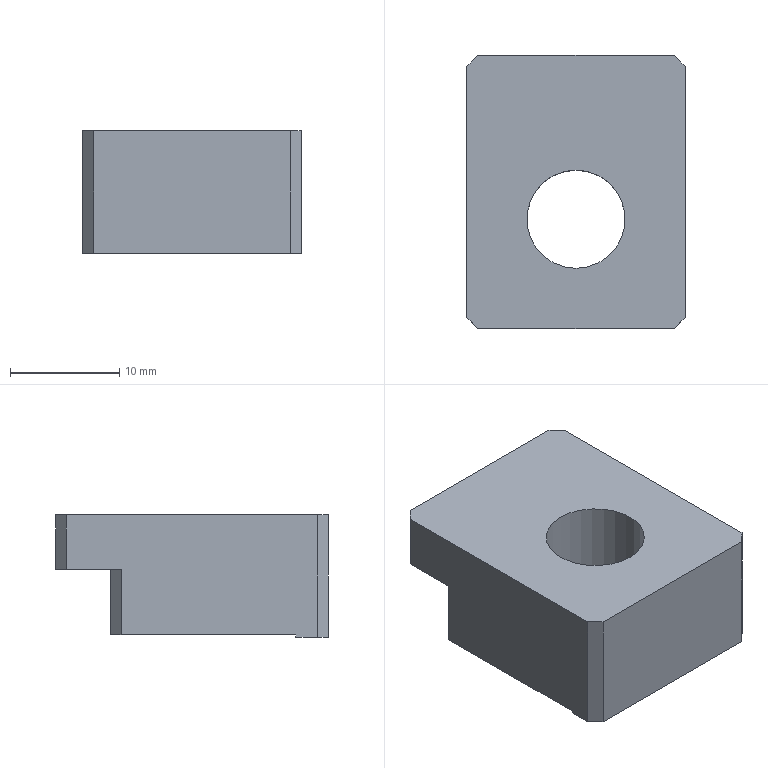Part | NX | features solid 2 | 1 solid | 17 faces | box 20 x 25 x 11.2 mm | volume 4190 mm3 | plane 16 | cylinder 1 | commonest cylinder face diameters 9 x1
STEP:
#1=CARTESIAN_POINT('',(146.5,-346.,61.));
#2=VERTEX_POINT('',#1);
#3=CARTESIAN_POINT('',(146.5,-350.5,61.));
#4=DIRECTION('',(0.,0.,-1.));
#5=DIRECTION('',(0.,1.,0.));
#6=AXIS2_PLACEMENT_3D('',#3,#4,#5);
#7=CIRCLE('',#6,4.5);
#8=EDGE_CURVE('',#2,#2,#7,.T.);
#9=ORIENTED_EDGE('',*,*,#8,.F.);
#10=EDGE_LOOP('',(#9));
#11=FACE_BOUND('',#10,.T.);
#12=CARTESIAN_POINT('',(146.5,-355.,50.));
#13=VERTEX_POINT('',#12);
#14=CARTESIAN_POINT('',(146.5,-350.5,50.));
#15=DIRECTION('',(0.,0.,1.));
#16=DIRECTION('',(0.,-1.,0.));
#17=AXIS2_PLACEMENT_3D('',#14,#15,#16);
#18=CIRCLE('',#17,4.5);
#19=EDGE_CURVE('',#13,#13,#18,.T.);
#20=ORIENTED_EDGE('',*,*,#19,.F.);
#21=EDGE_LOOP('',(#20));
#22=FACE_BOUND('',#21,.T.);
#23=CARTESIAN_POINT('',(146.5,-350.5,10.));
#24=DIRECTION('',(0.,0.,-1.));
#25=DIRECTION('',(0.,1.,0.));
#26=AXIS2_PLACEMENT_3D('',#23,#24,#25);
#27=CYLINDRICAL_SURFACE('',#26,4.5);
#28=ADVANCED_FACE('',(#11,#22),#27,.F.);
#29=CARTESIAN_POINT('',(155.5,-335.5,61.));
#30=VERTEX_POINT('',#29);
#31=CARTESIAN_POINT('',(137.5,-335.5,61.));
#32=VERTEX_POINT('',#31);
#33=CARTESIAN_POINT('',(177.825,-335.5,61.));
#34=DIRECTION('',(-1.,0.,0.));
#35=VECTOR('',#34,1000.);
#36=LINE('',#33,#35);
#37=EDGE_CURVE('',#30,#32,#36,.T.);
#38=ORIENTED_EDGE('',*,*,#37,.T.);
#39=CARTESIAN_POINT('',(136.5,-336.5,61.));
#40=VERTEX_POINT('',#39);
#41=CARTESIAN_POINT('',(137.5,-335.5,61.));
#42=DIRECTION('',(-0.7071,-0.7071,0.));
#43=VECTOR('',#42,1000.);
#44=LINE('',#41,#43);
#45=EDGE_CURVE('',#32,#40,#44,.T.);
#46=ORIENTED_EDGE('',*,*,#45,.T.);
#47=CARTESIAN_POINT('',(136.5,-359.5,61.));
#48=VERTEX_POINT('',#47);
#49=CARTESIAN_POINT('',(136.5,-323.825,61.));
#50=DIRECTION('',(0.,1.,0.));
#51=VECTOR('',#50,1000.);
#52=LINE('',#49,#51);
#53=EDGE_CURVE('',#48,#40,#52,.T.);
#54=ORIENTED_EDGE('',*,*,#53,.F.);
#55=CARTESIAN_POINT('',(137.5,-360.5,61.));
#56=VERTEX_POINT('',#55);
#57=CARTESIAN_POINT('',(136.5,-359.5,61.));
#58=DIRECTION('',(0.7071,-0.7071,0.));
#59=VECTOR('',#58,1000.);
#60=LINE('',#57,#59);
#61=EDGE_CURVE('',#48,#56,#60,.T.);
#62=ORIENTED_EDGE('',*,*,#61,.T.);
#63=CARTESIAN_POINT('',(155.5,-360.5,61.));
#64=VERTEX_POINT('',#63);
#65=CARTESIAN_POINT('',(177.825,-360.5,61.));
#66=DIRECTION('',(1.,0.,0.));
#67=VECTOR('',#66,1000.);
#68=LINE('',#65,#67);
#69=EDGE_CURVE('',#56,#64,#68,.T.);
#70=ORIENTED_EDGE('',*,*,#69,.T.);
#71=CARTESIAN_POINT('',(156.5,-359.5,61.));
#72=VERTEX_POINT('',#71);
#73=CARTESIAN_POINT('',(155.5,-360.5,61.));
#74=DIRECTION('',(0.7071,0.7071,0.));
#75=VECTOR('',#74,1000.);
#76=LINE('',#73,#75);
#77=EDGE_CURVE('',#64,#72,#76,.T.);
#78=ORIENTED_EDGE('',*,*,#77,.T.);
#79=CARTESIAN_POINT('',(156.5,-336.5,61.));
#80=VERTEX_POINT('',#79);
#81=CARTESIAN_POINT('',(156.5,-323.825,61.));
#82=DIRECTION('',(0.,1.,0.));
#83=VECTOR('',#82,1000.);
#84=LINE('',#81,#83);
#85=EDGE_CURVE('',#72,#80,#84,.T.);
#86=ORIENTED_EDGE('',*,*,#85,.T.);
#87=CARTESIAN_POINT('',(155.5,-335.5,61.));
#88=DIRECTION('',(-0.7071,0.7071,0.));
#89=VECTOR('',#88,1000.);
#90=LINE('',#87,#89);
#91=EDGE_CURVE('',#80,#30,#90,.T.);
#92=ORIENTED_EDGE('',*,*,#91,.T.);
#93=EDGE_LOOP('',(#38,#46,#54,#62,#70,#78,#86,#92));
#94=FACE_BOUND('',#93,.T.);
#95=ORIENTED_EDGE('',*,*,#8,.T.);
#96=EDGE_LOOP('',(#95));
#97=FACE_BOUND('',#96,.T.);
#98=CARTESIAN_POINT('',(177.825,-323.825,61.));
#99=DIRECTION('',(0.,0.,-1.));
#100=DIRECTION('',(-0.7071,0.7071,0.));
#101=AXIS2_PLACEMENT_3D('',#98,#99,#100);
#102=PLANE('',#101);
#103=ADVANCED_FACE('',(#94,#97),#102,.F.);
#104=ORIENTED_EDGE('',*,*,#91,.F.);
#105=CARTESIAN_POINT('',(156.5,-336.5,56.));
#106=VERTEX_POINT('',#105);
#107=CARTESIAN_POINT('',(156.5,-336.5,57.5));
#108=DIRECTION('',(0.,0.,1.));
#109=VECTOR('',#108,1000.);
#110=LINE('',#107,#109);
#111=EDGE_CURVE('',#106,#80,#110,.T.);
#112=ORIENTED_EDGE('',*,*,#111,.F.);
#113=CARTESIAN_POINT('',(155.5,-335.5,56.));
#114=VERTEX_POINT('',#113);
#115=CARTESIAN_POINT('',(155.5,-335.5,56.));
#116=DIRECTION('',(0.7071,-0.7071,0.));
#117=VECTOR('',#116,1000.);
#118=LINE('',#115,#117);
#119=EDGE_CURVE('',#114,#106,#118,.T.);
#120=ORIENTED_EDGE('',*,*,#119,.F.);
#121=CARTESIAN_POINT('',(155.5,-335.5,60.));
#122=DIRECTION('',(0.,0.,-1.));
#123=VECTOR('',#122,1000.);
#124=LINE('',#121,#123);
#125=EDGE_CURVE('',#30,#114,#124,.T.);
#126=ORIENTED_EDGE('',*,*,#125,.F.);
#127=EDGE_LOOP('',(#104,#112,#120,#126));
#128=FACE_BOUND('',#127,.T.);
#129=CARTESIAN_POINT('',(155.5,-335.5,60.));
#130=DIRECTION('',(-0.7071,-0.7071,0.));
#131=DIRECTION('',(0.,0.,-1.));
#132=AXIS2_PLACEMENT_3D('',#129,#130,#131);
#133=PLANE('',#132);
#134=ADVANCED_FACE('',(#128),#133,.F.);
#135=CARTESIAN_POINT('',(136.5,-336.5,56.));
#136=VERTEX_POINT('',#135);
#137=CARTESIAN_POINT('',(137.5,-335.5,56.));
#138=VERTEX_POINT('',#137);
#139=CARTESIAN_POINT('',(137.5,-335.5,56.));
#140=DIRECTION('',(0.7071,0.7071,0.));
#141=VECTOR('',#140,1000.);
#142=LINE('',#139,#141);
#143=EDGE_CURVE('',#136,#138,#142,.T.);
#144=ORIENTED_EDGE('',*,*,#143,.F.);
#145=CARTESIAN_POINT('',(136.5,-336.5,56.3));
#146=DIRECTION('',(0.,0.,-1.));
#147=VECTOR('',#146,1000.);
#148=LINE('',#145,#147);
#149=EDGE_CURVE('',#40,#136,#148,.T.);
#150=ORIENTED_EDGE('',*,*,#149,.F.);
#151=ORIENTED_EDGE('',*,*,#45,.F.);
#152=CARTESIAN_POINT('',(137.5,-335.5,64.8));
#153=DIRECTION('',(0.,0.,1.));
#154=VECTOR('',#153,1000.);
#155=LINE('',#152,#154);
#156=EDGE_CURVE('',#138,#32,#155,.T.);
#157=ORIENTED_EDGE('',*,*,#156,.F.);
#158=EDGE_LOOP('',(#144,#150,#151,#157));
#159=FACE_BOUND('',#158,.T.);
#160=CARTESIAN_POINT('',(137.5,-335.5,60.));
#161=DIRECTION('',(-0.7071,0.7071,0.));
#162=DIRECTION('',(0.,0.,-1.));
#163=AXIS2_PLACEMENT_3D('',#160,#161,#162);
#164=PLANE('',#163);
#165=ADVANCED_FACE('',(#159),#164,.T.);
#166=CARTESIAN_POINT('',(140.,-335.5,56.));
#167=DIRECTION('',(1.,0.,0.));
#168=VECTOR('',#167,1000.);
#169=LINE('',#166,#168);
#170=EDGE_CURVE('',#138,#114,#169,.T.);
#171=ORIENTED_EDGE('',*,*,#170,.F.);
#172=ORIENTED_EDGE('',*,*,#156,.T.);
#173=ORIENTED_EDGE('',*,*,#37,.F.);
#174=ORIENTED_EDGE('',*,*,#125,.T.);
#175=EDGE_LOOP('',(#171,#172,#173,#174));
#176=FACE_BOUND('',#175,.T.);
#177=CARTESIAN_POINT('',(136.,-335.5,60.));
#178=DIRECTION('',(0.,-1.,0.));
#179=DIRECTION('',(0.,0.,-1.));
#180=AXIS2_PLACEMENT_3D('',#177,#178,#179);
#181=PLANE('',#180);
#182=ADVANCED_FACE('',(#176),#181,.F.);
#183=CARTESIAN_POINT('',(156.5,-341.5,56.));
#184=VERTEX_POINT('',#183);
#185=CARTESIAN_POINT('',(156.5,-343.5,56.));
#186=DIRECTION('',(0.,-1.,0.));
#187=VECTOR('',#186,1000.);
#188=LINE('',#185,#187);
#189=EDGE_CURVE('',#106,#184,#188,.T.);
#190=ORIENTED_EDGE('',*,*,#189,.T.);
#191=CARTESIAN_POINT('',(155.5,-340.5,56.));
#192=VERTEX_POINT('',#191);
#193=CARTESIAN_POINT('',(148.,-333.,56.));
#194=DIRECTION('',(-0.7071,0.7071,0.));
#195=VECTOR('',#194,1000.);
#196=LINE('',#193,#195);
#197=EDGE_CURVE('',#184,#192,#196,.T.);
#198=ORIENTED_EDGE('',*,*,#197,.T.);
#199=CARTESIAN_POINT('',(137.5,-340.5,56.));
#200=VERTEX_POINT('',#199);
#201=CARTESIAN_POINT('',(140.,-340.5,56.));
#202=DIRECTION('',(-1.,0.,0.));
#203=VECTOR('',#202,1000.);
#204=LINE('',#201,#203);
#205=EDGE_CURVE('',#192,#200,#204,.T.);
#206=ORIENTED_EDGE('',*,*,#205,.T.);
#207=CARTESIAN_POINT('',(136.5,-341.5,56.));
#208=VERTEX_POINT('',#207);
#209=CARTESIAN_POINT('',(138.5,-339.5,56.));
#210=DIRECTION('',(-0.7071,-0.7071,0.));
#211=VECTOR('',#210,1000.);
#212=LINE('',#209,#211);
#213=EDGE_CURVE('',#200,#208,#212,.T.);
#214=ORIENTED_EDGE('',*,*,#213,.T.);
#215=CARTESIAN_POINT('',(136.5,-341.5,56.));
#216=DIRECTION('',(0.,1.,0.));
#217=VECTOR('',#216,1000.);
#218=LINE('',#215,#217);
#219=EDGE_CURVE('',#208,#136,#218,.T.);
#220=ORIENTED_EDGE('',*,*,#219,.T.);
#221=ORIENTED_EDGE('',*,*,#143,.T.);
#222=ORIENTED_EDGE('',*,*,#170,.T.);
#223=ORIENTED_EDGE('',*,*,#119,.T.);
#224=EDGE_LOOP('',(#190,#198,#206,#214,#220,#221,#222,#223));
#225=FACE_BOUND('',#224,.T.);
#226=CARTESIAN_POINT('',(140.,-343.5,56.));
#227=DIRECTION('',(0.,0.,1.));
#228=DIRECTION('',(0.,-1.,0.));
#229=AXIS2_PLACEMENT_3D('',#226,#227,#228);
#230=PLANE('',#229);
#231=ADVANCED_FACE('',(#225),#230,.F.);
#232=CARTESIAN_POINT('',(155.5,-360.5,49.8));
#233=VERTEX_POINT('',#232);
#234=CARTESIAN_POINT('',(155.5,-360.5,51.5));
#235=DIRECTION('',(0.,0.,1.));
#236=VECTOR('',#235,1000.);
#237=LINE('',#234,#236);
#238=EDGE_CURVE('',#233,#64,#237,.T.);
#239=ORIENTED_EDGE('',*,*,#238,.F.);
#240=CARTESIAN_POINT('',(156.5,-359.5,49.8));
#241=VERTEX_POINT('',#240);
#242=CARTESIAN_POINT('',(155.5,-360.5,49.8));
#243=DIRECTION('',(-0.7071,-0.7071,0.));
#244=VECTOR('',#243,1000.);
#245=LINE('',#242,#244);
#246=EDGE_CURVE('',#241,#233,#245,.T.);
#247=ORIENTED_EDGE('',*,*,#246,.F.);
#248=CARTESIAN_POINT('',(156.5,-359.5,57.5));
#249=DIRECTION('',(0.,0.,-1.));
#250=VECTOR('',#249,1000.);
#251=LINE('',#248,#250);
#252=EDGE_CURVE('',#72,#241,#251,.T.);
#253=ORIENTED_EDGE('',*,*,#252,.F.);
#254=ORIENTED_EDGE('',*,*,#77,.F.);
#255=EDGE_LOOP('',(#239,#247,#253,#254));
#256=FACE_BOUND('',#255,.T.);
#257=CARTESIAN_POINT('',(155.5,-360.5,51.5));
#258=DIRECTION('',(-0.7071,0.7071,0.));
#259=DIRECTION('',(0.,0.,1.));
#260=AXIS2_PLACEMENT_3D('',#257,#258,#259);
#261=PLANE('',#260);
#262=ADVANCED_FACE('',(#256),#261,.F.);
#263=ORIENTED_EDGE('',*,*,#252,.T.);
#264=CARTESIAN_POINT('',(156.5,-357.5,49.8));
#265=VERTEX_POINT('',#264);
#266=CARTESIAN_POINT('',(156.5,-348.5,49.8));
#267=DIRECTION('',(0.,-1.,0.));
#268=VECTOR('',#267,1000.);
#269=LINE('',#266,#268);
#270=EDGE_CURVE('',#265,#241,#269,.T.);
#271=ORIENTED_EDGE('',*,*,#270,.F.);
#272=CARTESIAN_POINT('',(156.5,-357.5,50.));
#273=VERTEX_POINT('',#272);
#274=CARTESIAN_POINT('',(156.5,-357.5,57.5));
#275=DIRECTION('',(0.,0.,1.));
#276=VECTOR('',#275,1000.);
#277=LINE('',#274,#276);
#278=EDGE_CURVE('',#265,#273,#277,.T.);
#279=ORIENTED_EDGE('',*,*,#278,.T.);
#280=CARTESIAN_POINT('',(156.5,-341.5,50.));
#281=VERTEX_POINT('',#280);
#282=CARTESIAN_POINT('',(156.5,-343.5,50.));
#283=DIRECTION('',(0.,-1.,0.));
#284=VECTOR('',#283,1000.);
#285=LINE('',#282,#284);
#286=EDGE_CURVE('',#281,#273,#285,.T.);
#287=ORIENTED_EDGE('',*,*,#286,.F.);
#288=CARTESIAN_POINT('',(156.5,-341.5,57.5));
#289=DIRECTION('',(0.,0.,1.));
#290=VECTOR('',#289,1000.);
#291=LINE('',#288,#290);
#292=EDGE_CURVE('',#281,#184,#291,.T.);
#293=ORIENTED_EDGE('',*,*,#292,.T.);
#294=ORIENTED_EDGE('',*,*,#189,.F.);
#295=ORIENTED_EDGE('',*,*,#111,.T.);
#296=ORIENTED_EDGE('',*,*,#85,.F.);
#297=EDGE_LOOP('',(#263,#271,#279,#287,#293,#294,#295,#296));
#298=FACE_BOUND('',#297,.T.);
#299=CARTESIAN_POINT('',(156.5,-341.5,57.5));
#300=DIRECTION('',(-1.,0.,0.));
#301=DIRECTION('',(0.,0.,-1.));
#302=AXIS2_PLACEMENT_3D('',#299,#300,#301);
#303=PLANE('',#302);
#304=ADVANCED_FACE('',(#298),#303,.F.);
#305=CARTESIAN_POINT('',(136.5,-359.5,49.8));
#306=VERTEX_POINT('',#305);
#307=CARTESIAN_POINT('',(136.5,-359.5,64.8));
#308=DIRECTION('',(0.,0.,1.));
#309=VECTOR('',#308,1000.);
#310=LINE('',#307,#309);
#311=EDGE_CURVE('',#306,#48,#310,.T.);
#312=ORIENTED_EDGE('',*,*,#311,.F.);
#313=CARTESIAN_POINT('',(137.5,-360.5,49.8));
#314=VERTEX_POINT('',#313);
#315=CARTESIAN_POINT('',(136.5,-359.5,49.8));
#316=DIRECTION('',(-0.7071,0.7071,0.));
#317=VECTOR('',#316,1000.);
#318=LINE('',#315,#317);
#319=EDGE_CURVE('',#314,#306,#318,.T.);
#320=ORIENTED_EDGE('',*,*,#319,.F.);
#321=CARTESIAN_POINT('',(137.5,-360.5,49.8));
#322=DIRECTION('',(0.,0.,-1.));
#323=VECTOR('',#322,1000.);
#324=LINE('',#321,#323);
#325=EDGE_CURVE('',#56,#314,#324,.T.);
#326=ORIENTED_EDGE('',*,*,#325,.F.);
#327=ORIENTED_EDGE('',*,*,#61,.F.);
#328=EDGE_LOOP('',(#312,#320,#326,#327));
#329=FACE_BOUND('',#328,.T.);
#330=CARTESIAN_POINT('',(136.5,-359.5,57.5));
#331=DIRECTION('',(-0.7071,-0.7071,0.));
#332=DIRECTION('',(0.,0.,-1.));
#333=AXIS2_PLACEMENT_3D('',#330,#331,#332);
#334=PLANE('',#333);
#335=ADVANCED_FACE('',(#329),#334,.T.);
#336=ORIENTED_EDGE('',*,*,#219,.F.);
#337=CARTESIAN_POINT('',(136.5,-341.5,50.));
#338=VERTEX_POINT('',#337);
#339=CARTESIAN_POINT('',(136.5,-341.5,50.));
#340=DIRECTION('',(0.,0.,-1.));
#341=VECTOR('',#340,1000.);
#342=LINE('',#339,#341);
#343=EDGE_CURVE('',#208,#338,#342,.T.);
#344=ORIENTED_EDGE('',*,*,#343,.T.);
#345=CARTESIAN_POINT('',(136.5,-357.5,50.));
#346=VERTEX_POINT('',#345);
#347=CARTESIAN_POINT('',(136.5,-343.5,50.));
#348=DIRECTION('',(0.,-1.,0.));
#349=VECTOR('',#348,1000.);
#350=LINE('',#347,#349);
#351=EDGE_CURVE('',#338,#346,#350,.T.);
#352=ORIENTED_EDGE('',*,*,#351,.T.);
#353=CARTESIAN_POINT('',(136.5,-357.5,49.8));
#354=VERTEX_POINT('',#353);
#355=CARTESIAN_POINT('',(136.5,-357.5,57.5));
#356=DIRECTION('',(0.,0.,1.));
#357=VECTOR('',#356,1000.);
#358=LINE('',#355,#357);
#359=EDGE_CURVE('',#354,#346,#358,.T.);
#360=ORIENTED_EDGE('',*,*,#359,.F.);
#361=CARTESIAN_POINT('',(136.5,-348.5,49.8));
#362=DIRECTION('',(0.,-1.,0.));
#363=VECTOR('',#362,1000.);
#364=LINE('',#361,#363);
#365=EDGE_CURVE('',#354,#306,#364,.T.);
#366=ORIENTED_EDGE('',*,*,#365,.T.);
#367=ORIENTED_EDGE('',*,*,#311,.T.);
#368=ORIENTED_EDGE('',*,*,#53,.T.);
#369=ORIENTED_EDGE('',*,*,#149,.T.);
#370=EDGE_LOOP('',(#336,#344,#352,#360,#366,#367,#368,#369));
#371=FACE_BOUND('',#370,.T.);
#372=CARTESIAN_POINT('',(136.5,-341.5,57.5));
#373=DIRECTION('',(-1.,0.,0.));
#374=DIRECTION('',(0.,0.,-1.));
#375=AXIS2_PLACEMENT_3D('',#372,#373,#374);
#376=PLANE('',#375);
#377=ADVANCED_FACE('',(#371),#376,.T.);
#378=ORIENTED_EDGE('',*,*,#325,.T.);
#379=CARTESIAN_POINT('',(140.,-360.5,49.8));
#380=DIRECTION('',(1.,0.,0.));
#381=VECTOR('',#380,1000.);
#382=LINE('',#379,#381);
#383=EDGE_CURVE('',#314,#233,#382,.T.);
#384=ORIENTED_EDGE('',*,*,#383,.T.);
#385=ORIENTED_EDGE('',*,*,#238,.T.);
#386=ORIENTED_EDGE('',*,*,#69,.F.);
#387=EDGE_LOOP('',(#378,#384,#385,#386));
#388=FACE_BOUND('',#387,.T.);
#389=CARTESIAN_POINT('',(140.,-360.5,51.5));
#390=DIRECTION('',(0.,1.,0.));
#391=DIRECTION('',(0.,0.,1.));
#392=AXIS2_PLACEMENT_3D('',#389,#390,#391);
#393=PLANE('',#392);
#394=ADVANCED_FACE('',(#388),#393,.F.);
#395=ORIENTED_EDGE('',*,*,#359,.T.);
#396=CARTESIAN_POINT('',(140.,-357.5,50.));
#397=DIRECTION('',(1.,0.,0.));
#398=VECTOR('',#397,1000.);
#399=LINE('',#396,#398);
#400=EDGE_CURVE('',#346,#273,#399,.T.);
#401=ORIENTED_EDGE('',*,*,#400,.T.);
#402=ORIENTED_EDGE('',*,*,#278,.F.);
#403=CARTESIAN_POINT('',(140.,-357.5,49.8));
#404=DIRECTION('',(1.,0.,0.));
#405=VECTOR('',#404,1000.);
#406=LINE('',#403,#405);
#407=EDGE_CURVE('',#354,#265,#406,.T.);
#408=ORIENTED_EDGE('',*,*,#407,.F.);
#409=EDGE_LOOP('',(#395,#401,#402,#408));
#410=FACE_BOUND('',#409,.T.);
#411=CARTESIAN_POINT('',(146.5,-357.5,55.75));
#412=DIRECTION('',(0.,-1.,0.));
#413=DIRECTION('',(0.,0.,-1.));
#414=AXIS2_PLACEMENT_3D('',#411,#412,#413);
#415=PLANE('',#414);
#416=ADVANCED_FACE('',(#410),#415,.F.);
#417=ORIENTED_EDGE('',*,*,#383,.F.);
#418=ORIENTED_EDGE('',*,*,#319,.T.);
#419=ORIENTED_EDGE('',*,*,#365,.F.);
#420=ORIENTED_EDGE('',*,*,#407,.T.);
#421=ORIENTED_EDGE('',*,*,#270,.T.);
#422=ORIENTED_EDGE('',*,*,#246,.T.);
#423=EDGE_LOOP('',(#417,#418,#419,#420,#421,#422));
#424=FACE_BOUND('',#423,.T.);
#425=CARTESIAN_POINT('',(140.,-348.5,49.8));
#426=DIRECTION('',(0.,0.,1.));
#427=DIRECTION('',(0.,-1.,0.));
#428=AXIS2_PLACEMENT_3D('',#425,#426,#427);
#429=PLANE('',#428);
#430=ADVANCED_FACE('',(#424),#429,.F.);
#431=ORIENTED_EDGE('',*,*,#351,.F.);
#432=CARTESIAN_POINT('',(137.5,-340.5,50.));
#433=VERTEX_POINT('',#432);
#434=CARTESIAN_POINT('',(136.5,-341.5,50.));
#435=DIRECTION('',(0.7071,0.7071,0.));
#436=VECTOR('',#435,1000.);
#437=LINE('',#434,#436);
#438=EDGE_CURVE('',#338,#433,#437,.T.);
#439=ORIENTED_EDGE('',*,*,#438,.T.);
#440=CARTESIAN_POINT('',(155.5,-340.5,50.));
#441=VERTEX_POINT('',#440);
#442=CARTESIAN_POINT('',(140.,-340.5,50.));
#443=DIRECTION('',(1.,0.,0.));
#444=VECTOR('',#443,1000.);
#445=LINE('',#442,#444);
#446=EDGE_CURVE('',#433,#441,#445,.T.);
#447=ORIENTED_EDGE('',*,*,#446,.T.);
#448=CARTESIAN_POINT('',(155.5,-340.5,50.));
#449=DIRECTION('',(0.7071,-0.7071,0.));
#450=VECTOR('',#449,1000.);
#451=LINE('',#448,#450);
#452=EDGE_CURVE('',#441,#281,#451,.T.);
#453=ORIENTED_EDGE('',*,*,#452,.T.);
#454=ORIENTED_EDGE('',*,*,#286,.T.);
#455=ORIENTED_EDGE('',*,*,#400,.F.);
#456=EDGE_LOOP('',(#431,#439,#447,#453,#454,#455));
#457=FACE_BOUND('',#456,.T.);
#458=ORIENTED_EDGE('',*,*,#19,.T.);
#459=EDGE_LOOP('',(#458));
#460=FACE_BOUND('',#459,.T.);
#461=CARTESIAN_POINT('',(140.,-343.5,50.));
#462=DIRECTION('',(0.,0.,1.));
#463=DIRECTION('',(0.,-1.,0.));
#464=AXIS2_PLACEMENT_3D('',#461,#462,#463);
#465=PLANE('',#464);
#466=ADVANCED_FACE('',(#457,#460),#465,.F.);
#467=ORIENTED_EDGE('',*,*,#197,.F.);
#468=ORIENTED_EDGE('',*,*,#292,.F.);
#469=ORIENTED_EDGE('',*,*,#452,.F.);
#470=CARTESIAN_POINT('',(155.5,-340.5,57.5));
#471=DIRECTION('',(0.,0.,-1.));
#472=VECTOR('',#471,1000.);
#473=LINE('',#470,#472);
#474=EDGE_CURVE('',#192,#441,#473,.T.);
#475=ORIENTED_EDGE('',*,*,#474,.F.);
#476=EDGE_LOOP('',(#467,#468,#469,#475));
#477=FACE_BOUND('',#476,.T.);
#478=CARTESIAN_POINT('',(155.5,-340.5,57.5));
#479=DIRECTION('',(-0.7071,-0.7071,0.));
#480=DIRECTION('',(0.,0.,-1.));
#481=AXIS2_PLACEMENT_3D('',#478,#479,#480);
#482=PLANE('',#481);
#483=ADVANCED_FACE('',(#477),#482,.F.);
#484=ORIENTED_EDGE('',*,*,#213,.F.);
#485=CARTESIAN_POINT('',(137.5,-340.5,56.3));
#486=DIRECTION('',(0.,0.,1.));
#487=VECTOR('',#486,1000.);
#488=LINE('',#485,#487);
#489=EDGE_CURVE('',#433,#200,#488,.T.);
#490=ORIENTED_EDGE('',*,*,#489,.F.);
#491=ORIENTED_EDGE('',*,*,#438,.F.);
#492=ORIENTED_EDGE('',*,*,#343,.F.);
#493=EDGE_LOOP('',(#484,#490,#491,#492));
#494=FACE_BOUND('',#493,.T.);
#495=CARTESIAN_POINT('',(136.5,-341.5,57.5));
#496=DIRECTION('',(-0.7071,0.7071,0.));
#497=DIRECTION('',(0.,0.,1.));
#498=AXIS2_PLACEMENT_3D('',#495,#496,#497);
#499=PLANE('',#498);
#500=ADVANCED_FACE('',(#494),#499,.T.);
#501=ORIENTED_EDGE('',*,*,#446,.F.);
#502=ORIENTED_EDGE('',*,*,#489,.T.);
#503=ORIENTED_EDGE('',*,*,#205,.F.);
#504=ORIENTED_EDGE('',*,*,#474,.T.);
#505=EDGE_LOOP('',(#501,#502,#503,#504));
#506=FACE_BOUND('',#505,.T.);
#507=CARTESIAN_POINT('',(140.,-340.5,57.5));
#508=DIRECTION('',(0.,-1.,0.));
#509=DIRECTION('',(0.,0.,-1.));
#510=AXIS2_PLACEMENT_3D('',#507,#508,#509);
#511=PLANE('',#510);
#512=ADVANCED_FACE('',(#506),#511,.F.);
#513=CLOSED_SHELL('',(#28,#103,#134,#165,#182,#231,#262,#304,#335,#377,#394,#416,#430,#466,#483,#500,#512));
#514=MANIFOLD_SOLID_BREP('',#513);
#515=(LENGTH_UNIT()NAMED_UNIT(*)SI_UNIT(.MILLI.,.METRE.));
#516=UNCERTAINTY_MEASURE_WITH_UNIT(LENGTH_MEASURE(0.00001),#515,'','');
#517=(NAMED_UNIT(*)PLANE_ANGLE_UNIT()SI_UNIT($,.RADIAN.));
#518=(NAMED_UNIT(*)SI_UNIT($,.STERADIAN.)SOLID_ANGLE_UNIT());
#519=(GEOMETRIC_REPRESENTATION_CONTEXT(3)GLOBAL_UNCERTAINTY_ASSIGNED_CONTEXT((#516))GLOBAL_UNIT_ASSIGNED_CONTEXT((#515,#517,#518))REPRESENTATION_CONTEXT('',''));
#520=ADVANCED_BREP_SHAPE_REPRESENTATION('',(#514),#519);